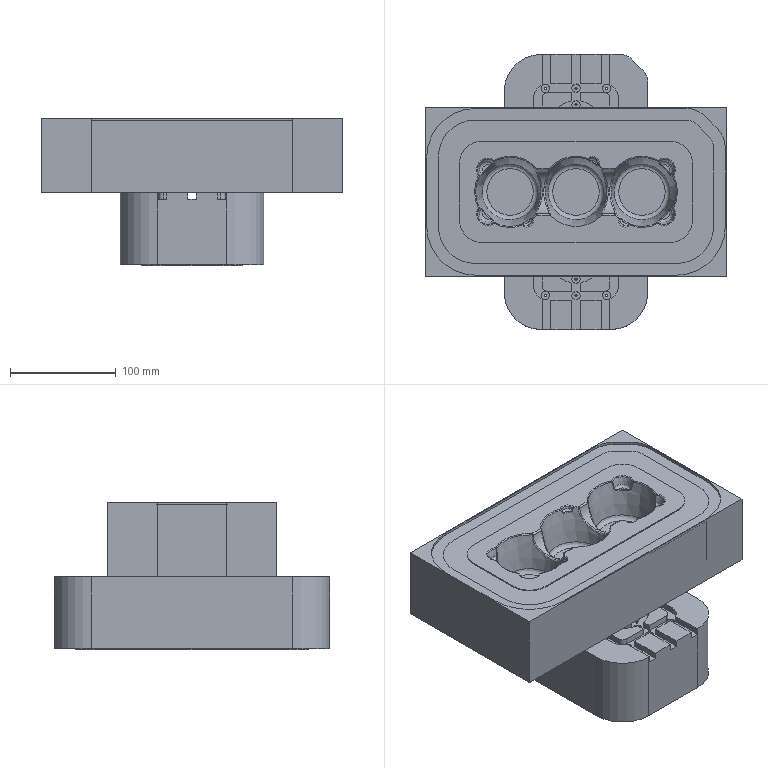NC program | NX | posted with a generic post | part box 284.317 x 260.317 x 139.5 mm
Lines 198434 to 198483 of 226982:
(DRILLING , TOOL : V2.0)
N396854 M6
N396856 G53
N396858 G17 G0 G90 X82.421 Y0. S2000 M3 M8
N396860 G43 Z220.5 H0
N396862 G94 G81 G98 Z27.603 F150. R32.603
N396864 X62.366 Y-20.055
N396866 Y0.
N396868 Y20.055
N396870 X42.311 Y0.
N396872 X20.055
N396874 X0. Y20.055
N396876 Y0.
N396878 Y-20.055
N396880 X-20.055 Y0.
N396882 X-62.366 Y-20.055
N396884 X-82.421 Y0.
N396886 X-62.366
N396888 Y20.055
N396890 X-42.311 Y0.
N396892 X-31.184 Z47.219 R52.219
N396894 Y18.667 Z61.212 R66.212
N396896 X-14.465 Y35.878 Z67. R72.
N396898 X-43.395
N396900 X-72.325
N396902 X-97.931 Y28.913
N396904 X-98.159 Y0.
N396906 X-97.931 Y-28.913
N396908 X-72.325 Y-35.878
N396910 X-43.395
N396912 X-31.184 Y-18.667 Z61.212 R66.212
N396914 X-14.465 Y-35.878 Z67. R72.
N396916 X14.465
N396918 X30.987 Y-18.667 Z61.212 R66.212
N396920 X43.395 Y-35.878 Z67. R72.
N396922 X72.325
N396924 X97.931 Y-28.913
N396926 X98.159 Y0.
N396928 X97.931 Y28.913
N396930 X72.325 Y35.878
N396932 X43.395
N396934 X14.465
N396936 X30.987 Y18.667 Z61.212 R66.212
N396938 Y0. Z47.219 R52.219
N396940 G80
N396942 G0 X30.987 Y0. Z220.5
N396944 M9
N396946 M5